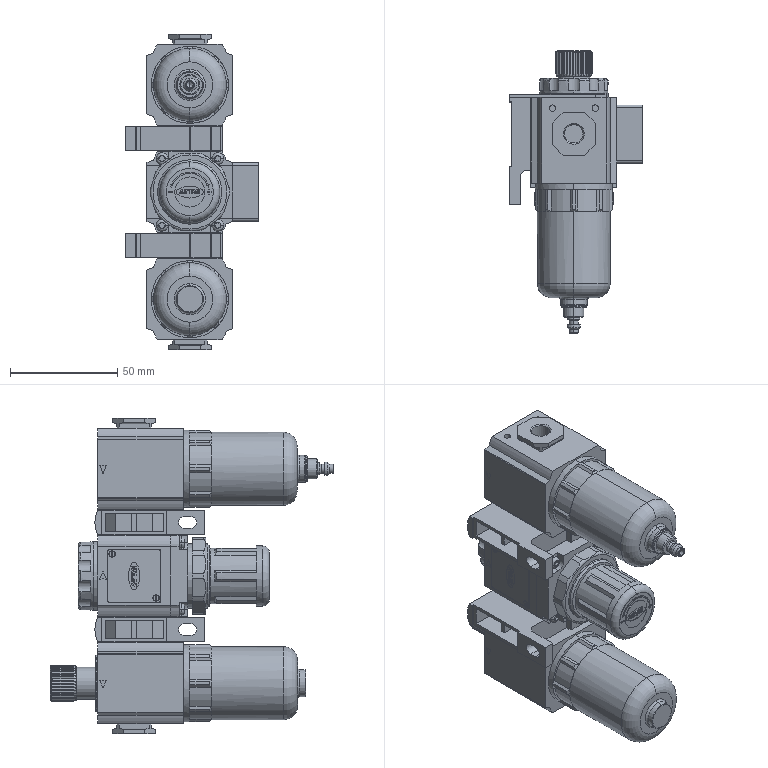Part | SolidWorks | 28 solids | 1798 faces | box 62 x 132 x 147 mm | volume 286848 mm3 | plane 1078 | cylinder 536 | cone 108 | torus 76 | commonest cylinder face diameters 3 x54 4 x28 0.4 x22 35.8 x18 6 x17 2.75 x16